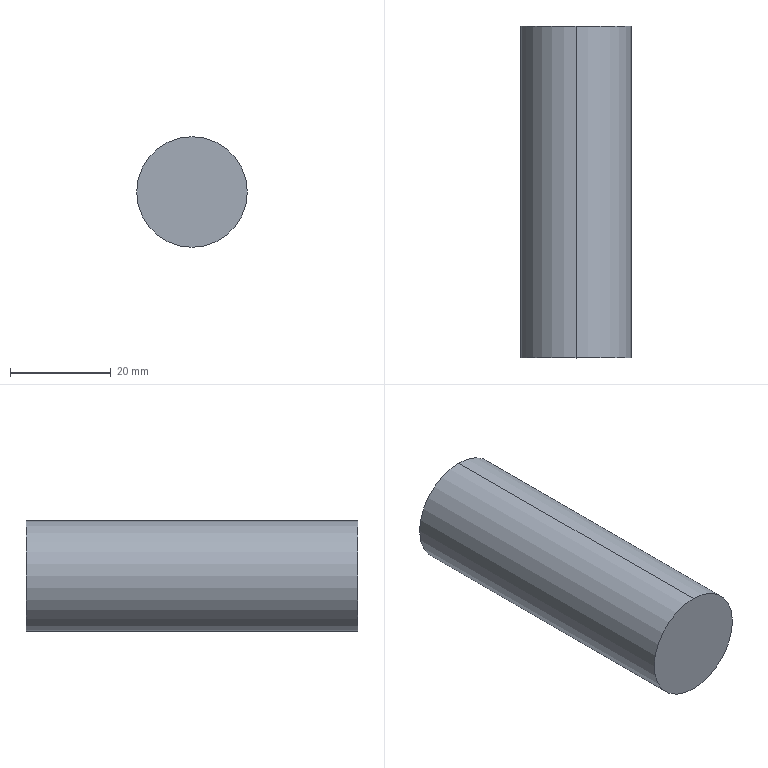Part | SolidWorks | features Extrusion 1, HoleWzd 1 | 1 solid | 8 faces | box 22 x 66 x 22 mm | volume 23622 mm3 | cylinder 4 | cone 2 | plane 2 | commonest cylinder face diameters 8.5 x2 22 x2
STEP:
#1=CARTESIAN_POINT('',(0.,41.,-4.25));
#2=VERTEX_POINT('',#1);
#3=CARTESIAN_POINT('',(0.,41.,4.25));
#4=VERTEX_POINT('',#3);
#5=CARTESIAN_POINT('',(0.,41.,0.));
#6=DIRECTION('',(0.,1.,0.));
#7=DIRECTION('',(0.,0.,1.));
#8=AXIS2_PLACEMENT_3D('',#5,#6,#7);
#9=CIRCLE('',#8,4.25);
#10=EDGE_CURVE('',#2,#4,#9,.T.);
#11=ORIENTED_EDGE('',*,*,#10,.F.);
#12=CARTESIAN_POINT('',(0.,66.,-4.25));
#13=VERTEX_POINT('',#12);
#14=CARTESIAN_POINT('',(0.,66.,-4.25));
#15=DIRECTION('',(0.,1.,0.));
#16=VECTOR('',#15,1000.);
#17=LINE('',#14,#16);
#18=EDGE_CURVE('',#2,#13,#17,.T.);
#19=ORIENTED_EDGE('',*,*,#18,.T.);
#20=CARTESIAN_POINT('',(0.,66.,4.25));
#21=VERTEX_POINT('',#20);
#22=CARTESIAN_POINT('',(0.,66.,0.));
#23=DIRECTION('',(0.,1.,0.));
#24=DIRECTION('',(0.,0.,1.));
#25=AXIS2_PLACEMENT_3D('',#22,#23,#24);
#26=CIRCLE('',#25,4.25);
#27=EDGE_CURVE('',#13,#21,#26,.T.);
#28=ORIENTED_EDGE('',*,*,#27,.T.);
#29=CARTESIAN_POINT('',(0.,66.,4.25));
#30=DIRECTION('',(0.,1.,0.));
#31=VECTOR('',#30,1000.);
#32=LINE('',#29,#31);
#33=EDGE_CURVE('',#4,#21,#32,.T.);
#34=ORIENTED_EDGE('',*,*,#33,.F.);
#35=EDGE_LOOP('',(#11,#19,#28,#34));
#36=FACE_OUTER_BOUND('',#35,.T.);
#37=CARTESIAN_POINT('',(0.,66.,0.));
#38=DIRECTION('',(0.,1.,0.));
#39=DIRECTION('',(0.,0.,1.));
#40=AXIS2_PLACEMENT_3D('',#37,#38,#39);
#41=CYLINDRICAL_SURFACE('',#40,4.25);
#42=ADVANCED_FACE('',(#36),#41,.F.);
#43=CARTESIAN_POINT('',(0.,38.446,0.));
#44=VERTEX_POINT('',#43);
#45=CARTESIAN_POINT('',(0.,41.,4.25));
#46=DIRECTION('',(0.,0.515,0.8572));
#47=VECTOR('',#46,1000.);
#48=LINE('',#45,#47);
#49=EDGE_CURVE('',#44,#4,#48,.T.);
#50=ORIENTED_EDGE('',*,*,#49,.F.);
#51=CARTESIAN_POINT('',(0.,41.,-4.25));
#52=DIRECTION('',(0.,0.515,-0.8572));
#53=VECTOR('',#52,1000.);
#54=LINE('',#51,#53);
#55=EDGE_CURVE('',#44,#2,#54,.T.);
#56=ORIENTED_EDGE('',*,*,#55,.T.);
#57=ORIENTED_EDGE('',*,*,#10,.T.);
#58=EDGE_LOOP('',(#50,#56,#57));
#59=FACE_OUTER_BOUND('',#58,.T.);
#60=CARTESIAN_POINT('',(0.,41.,0.));
#61=DIRECTION('',(0.,1.,0.));
#62=DIRECTION('',(0.,0.,1.));
#63=AXIS2_PLACEMENT_3D('',#60,#61,#62);
#64=CONICAL_SURFACE('',#63,4.25,1.03);
#65=ADVANCED_FACE('',(#59),#64,.F.);
#66=CARTESIAN_POINT('',(0.,66.,11.));
#67=VERTEX_POINT('',#66);
#68=CARTESIAN_POINT('',(0.,66.,-11.));
#69=VERTEX_POINT('',#68);
#70=CARTESIAN_POINT('',(0.,66.,0.));
#71=DIRECTION('',(0.,1.,0.));
#72=DIRECTION('',(0.,0.,1.));
#73=AXIS2_PLACEMENT_3D('',#70,#71,#72);
#74=CIRCLE('',#73,11.);
#75=EDGE_CURVE('',#67,#69,#74,.T.);
#76=ORIENTED_EDGE('',*,*,#75,.F.);
#77=CARTESIAN_POINT('',(0.,0.,11.));
#78=VERTEX_POINT('',#77);
#79=CARTESIAN_POINT('',(0.,66.,11.));
#80=DIRECTION('',(0.,-1.,0.));
#81=VECTOR('',#80,1000.);
#82=LINE('',#79,#81);
#83=EDGE_CURVE('',#67,#78,#82,.T.);
#84=ORIENTED_EDGE('',*,*,#83,.T.);
#85=CARTESIAN_POINT('',(0.,0.,-11.));
#86=VERTEX_POINT('',#85);
#87=CARTESIAN_POINT('',(0.,0.,0.));
#88=DIRECTION('',(0.,1.,0.));
#89=DIRECTION('',(0.,0.,1.));
#90=AXIS2_PLACEMENT_3D('',#87,#88,#89);
#91=CIRCLE('',#90,11.);
#92=EDGE_CURVE('',#78,#86,#91,.T.);
#93=ORIENTED_EDGE('',*,*,#92,.T.);
#94=CARTESIAN_POINT('',(0.,66.,-11.));
#95=DIRECTION('',(0.,-1.,0.));
#96=VECTOR('',#95,1000.);
#97=LINE('',#94,#96);
#98=EDGE_CURVE('',#69,#86,#97,.T.);
#99=ORIENTED_EDGE('',*,*,#98,.F.);
#100=EDGE_LOOP('',(#76,#84,#93,#99));
#101=FACE_OUTER_BOUND('',#100,.T.);
#102=CARTESIAN_POINT('',(0.,66.,0.));
#103=DIRECTION('',(0.,-1.,0.));
#104=DIRECTION('',(0.,0.,-1.));
#105=AXIS2_PLACEMENT_3D('',#102,#103,#104);
#106=CYLINDRICAL_SURFACE('',#105,11.);
#107=ADVANCED_FACE('',(#101),#106,.T.);
#108=ORIENTED_EDGE('',*,*,#83,.F.);
#109=CARTESIAN_POINT('',(0.,66.,0.));
#110=DIRECTION('',(0.,1.,0.));
#111=DIRECTION('',(0.,0.,1.));
#112=AXIS2_PLACEMENT_3D('',#109,#110,#111);
#113=CIRCLE('',#112,11.);
#114=EDGE_CURVE('',#69,#67,#113,.T.);
#115=ORIENTED_EDGE('',*,*,#114,.F.);
#116=ORIENTED_EDGE('',*,*,#98,.T.);
#117=CARTESIAN_POINT('',(0.,0.,0.));
#118=DIRECTION('',(0.,1.,0.));
#119=DIRECTION('',(0.,0.,1.));
#120=AXIS2_PLACEMENT_3D('',#117,#118,#119);
#121=CIRCLE('',#120,11.);
#122=EDGE_CURVE('',#86,#78,#121,.T.);
#123=ORIENTED_EDGE('',*,*,#122,.T.);
#124=EDGE_LOOP('',(#108,#115,#116,#123));
#125=FACE_OUTER_BOUND('',#124,.T.);
#126=CARTESIAN_POINT('',(0.,66.,0.));
#127=DIRECTION('',(0.,-1.,0.));
#128=DIRECTION('',(0.,0.,-1.));
#129=AXIS2_PLACEMENT_3D('',#126,#127,#128);
#130=CYLINDRICAL_SURFACE('',#129,11.);
#131=ADVANCED_FACE('',(#125),#130,.T.);
#132=CARTESIAN_POINT('',(0.,66.,0.));
#133=DIRECTION('',(0.,1.,0.));
#134=DIRECTION('',(0.,0.,1.));
#135=AXIS2_PLACEMENT_3D('',#132,#133,#134);
#136=CIRCLE('',#135,4.25);
#137=EDGE_CURVE('',#21,#13,#136,.T.);
#138=ORIENTED_EDGE('',*,*,#137,.F.);
#139=ORIENTED_EDGE('',*,*,#27,.F.);
#140=EDGE_LOOP('',(#138,#139));
#141=FACE_BOUND('',#140,.T.);
#142=ORIENTED_EDGE('',*,*,#114,.T.);
#143=ORIENTED_EDGE('',*,*,#75,.T.);
#144=EDGE_LOOP('',(#142,#143));
#145=FACE_OUTER_BOUND('',#144,.T.);
#146=CARTESIAN_POINT('',(0.,66.,0.));
#147=DIRECTION('',(0.,1.,0.));
#148=DIRECTION('',(0.,0.,1.));
#149=AXIS2_PLACEMENT_3D('',#146,#147,#148);
#150=PLANE('',#149);
#151=ADVANCED_FACE('',(#141,#145),#150,.T.);
#152=ORIENTED_EDGE('',*,*,#122,.F.);
#153=ORIENTED_EDGE('',*,*,#92,.F.);
#154=EDGE_LOOP('',(#152,#153));
#155=FACE_OUTER_BOUND('',#154,.T.);
#156=CARTESIAN_POINT('',(0.,0.,0.));
#157=DIRECTION('',(0.,1.,0.));
#158=DIRECTION('',(0.,0.,1.));
#159=AXIS2_PLACEMENT_3D('',#156,#157,#158);
#160=PLANE('',#159);
#161=ADVANCED_FACE('',(#155),#160,.F.);
#162=ORIENTED_EDGE('',*,*,#55,.F.);
#163=ORIENTED_EDGE('',*,*,#49,.T.);
#164=CARTESIAN_POINT('',(0.,41.,0.));
#165=DIRECTION('',(0.,1.,0.));
#166=DIRECTION('',(0.,0.,1.));
#167=AXIS2_PLACEMENT_3D('',#164,#165,#166);
#168=CIRCLE('',#167,4.25);
#169=EDGE_CURVE('',#4,#2,#168,.T.);
#170=ORIENTED_EDGE('',*,*,#169,.T.);
#171=EDGE_LOOP('',(#162,#163,#170));
#172=FACE_OUTER_BOUND('',#171,.T.);
#173=CARTESIAN_POINT('',(0.,41.,0.));
#174=DIRECTION('',(0.,1.,0.));
#175=DIRECTION('',(0.,0.,1.));
#176=AXIS2_PLACEMENT_3D('',#173,#174,#175);
#177=CONICAL_SURFACE('',#176,4.25,1.03);
#178=ADVANCED_FACE('',(#172),#177,.F.);
#179=ORIENTED_EDGE('',*,*,#18,.F.);
#180=ORIENTED_EDGE('',*,*,#169,.F.);
#181=ORIENTED_EDGE('',*,*,#33,.T.);
#182=ORIENTED_EDGE('',*,*,#137,.T.);
#183=EDGE_LOOP('',(#179,#180,#181,#182));
#184=FACE_OUTER_BOUND('',#183,.T.);
#185=CARTESIAN_POINT('',(0.,66.,0.));
#186=DIRECTION('',(0.,1.,0.));
#187=DIRECTION('',(0.,0.,1.));
#188=AXIS2_PLACEMENT_3D('',#185,#186,#187);
#189=CYLINDRICAL_SURFACE('',#188,4.25);
#190=ADVANCED_FACE('',(#184),#189,.F.);
#191=CLOSED_SHELL('',(#42,#65,#107,#131,#151,#161,#178,#190));
#192=MANIFOLD_SOLID_BREP('',#191);
#193=CARTESIAN_POINT('',(0.,0.,0.));
#194=DIRECTION('',(0.,0.,1.));
#195=DIRECTION('',(1.,0.,0.));
#196=AXIS2_PLACEMENT_3D('',#193,#194,#195);
#197=(LENGTH_UNIT()NAMED_UNIT(*)SI_UNIT(.MILLI.,.METRE.));
#198=UNCERTAINTY_MEASURE_WITH_UNIT(LENGTH_MEASURE(0.00001),#197,'','');
#199=(NAMED_UNIT(*)PLANE_ANGLE_UNIT()SI_UNIT($,.RADIAN.));
#200=(NAMED_UNIT(*)SI_UNIT($,.STERADIAN.)SOLID_ANGLE_UNIT());
#201=(GEOMETRIC_REPRESENTATION_CONTEXT(3)GLOBAL_UNCERTAINTY_ASSIGNED_CONTEXT((#198))GLOBAL_UNIT_ASSIGNED_CONTEXT((#197,#199,#200))REPRESENTATION_CONTEXT('',''));
#202=ADVANCED_BREP_SHAPE_REPRESENTATION('',(#192,#196),#201);